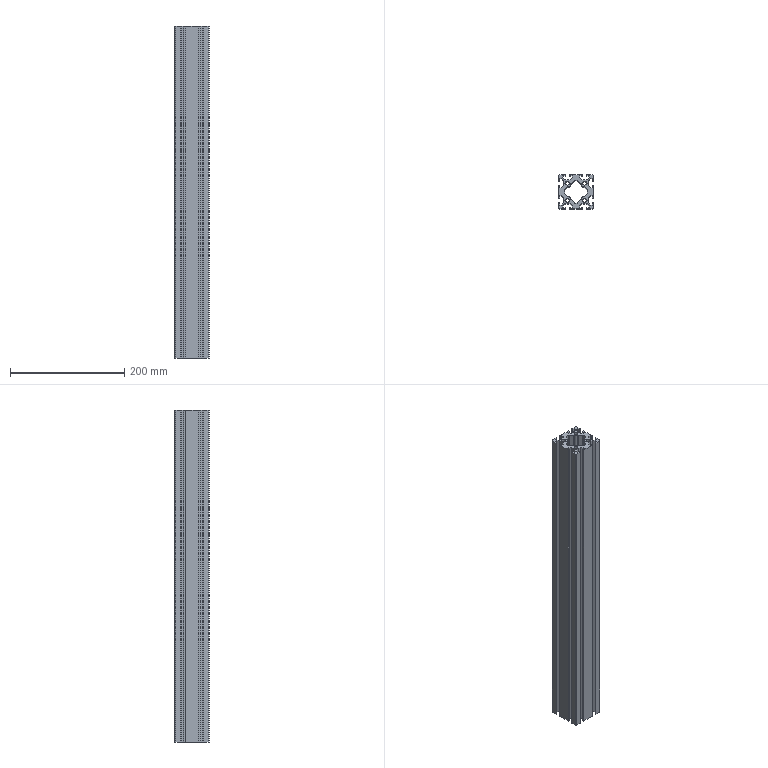Part | NX | features BREP 1 | 1 solid | 178 faces | box 60 x 60 x 580 mm | volume 886939 mm3 | plane 130 | cylinder 48 | commonest cylinder face diameters 0.6 x16 2 x16 6.8 x8 4 x4 6 x4